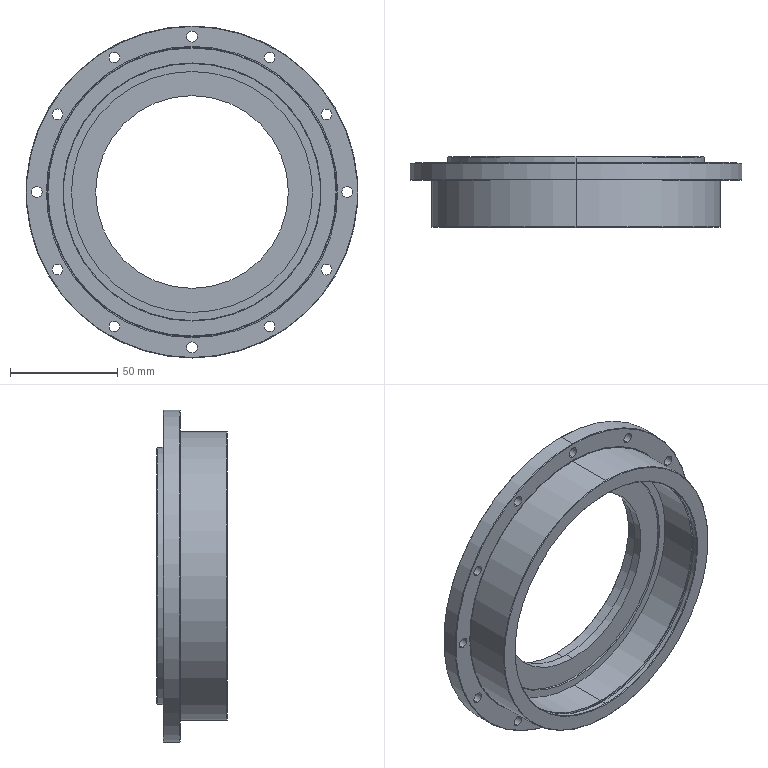Part | STEP file | 2026.6.15-Main Assembly图.sldasm-Part-127 | 1 solid | 66 faces | box 155 x 33 x 155 mm | volume 174909 mm3 | cylinder 44 | cone 12 | plane 10 | commonest cylinder face diameters 5 x24 120 x6 90 x2 95 x2 112.5 x2 121.5 x2